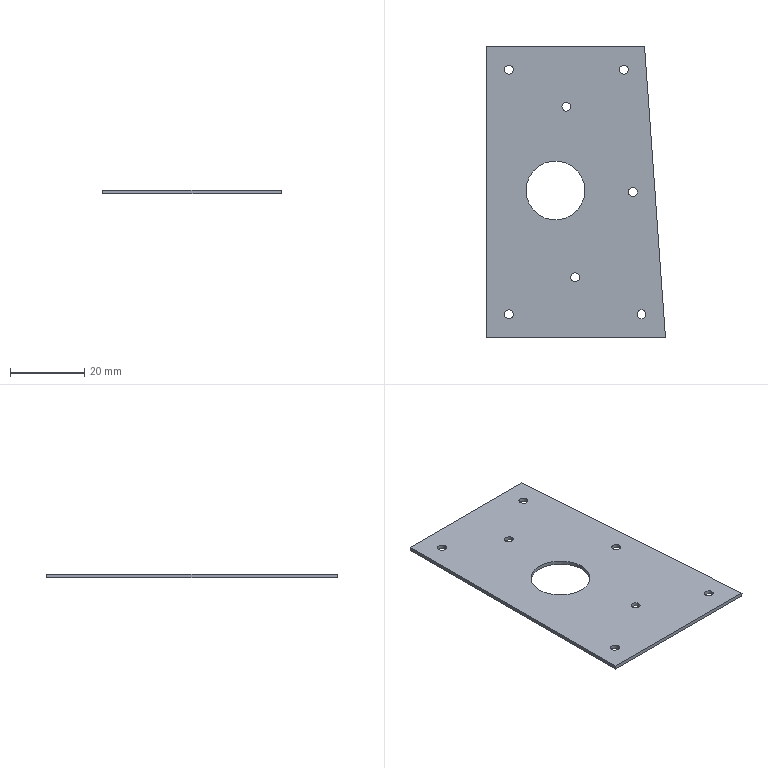Part | SolidWorks | features BaseBody 1 | 1 solid | 22 faces | box 48.271 x 78.4 x 1 mm | volume 3333 mm3 | cylinder 16 | plane 6 | commonest cylinder face diameters 2.4 x14 15.9 x2
STEP:
#1=CARTESIAN_POINT('',(26.55,40.,0.));
#2=VERTEX_POINT('',#1);
#3=CARTESIAN_POINT('',(10.65,40.,0.));
#4=VERTEX_POINT('',#3);
#5=CARTESIAN_POINT('',(18.6,40.,0.));
#6=DIRECTION('',(0.,0.,-1.));
#7=DIRECTION('',(1.,0.,0.));
#8=AXIS2_PLACEMENT_3D('',#5,#6,#7);
#9=CIRCLE('',#8,7.95);
#10=EDGE_CURVE('',#2,#4,#9,.T.);
#11=ORIENTED_EDGE('',*,*,#10,.T.);
#12=CARTESIAN_POINT('',(10.65,40.,1.));
#13=VERTEX_POINT('',#12);
#14=CARTESIAN_POINT('',(10.65,40.,0.));
#15=DIRECTION('',(0.,0.,1.));
#16=VECTOR('',#15,1000.);
#17=LINE('',#14,#16);
#18=EDGE_CURVE('',#4,#13,#17,.T.);
#19=ORIENTED_EDGE('',*,*,#18,.T.);
#20=CARTESIAN_POINT('',(26.55,40.,1.));
#21=VERTEX_POINT('',#20);
#22=CARTESIAN_POINT('',(18.6,40.,1.));
#23=DIRECTION('',(0.,0.,1.));
#24=DIRECTION('',(1.,0.,0.));
#25=AXIS2_PLACEMENT_3D('',#22,#23,#24);
#26=CIRCLE('',#25,7.95);
#27=EDGE_CURVE('',#13,#21,#26,.T.);
#28=ORIENTED_EDGE('',*,*,#27,.T.);
#29=CARTESIAN_POINT('',(26.55,40.,0.));
#30=DIRECTION('',(0.,0.,1.));
#31=VECTOR('',#30,1000.);
#32=LINE('',#29,#31);
#33=EDGE_CURVE('',#2,#21,#32,.T.);
#34=ORIENTED_EDGE('',*,*,#33,.F.);
#35=EDGE_LOOP('',(#11,#19,#28,#34));
#36=FACE_OUTER_BOUND('',#35,.T.);
#37=CARTESIAN_POINT('',(18.6,40.,0.));
#38=DIRECTION('',(0.,0.,1.));
#39=DIRECTION('',(1.,0.,0.));
#40=AXIS2_PLACEMENT_3D('',#37,#38,#39);
#41=CYLINDRICAL_SURFACE('',#40,7.95);
#42=ADVANCED_FACE('',(#36),#41,.F.);
#43=CARTESIAN_POINT('',(4.8,72.6,0.));
#44=VERTEX_POINT('',#43);
#45=CARTESIAN_POINT('',(7.2,72.6,0.));
#46=VERTEX_POINT('',#45);
#47=CARTESIAN_POINT('',(6.,72.6,0.));
#48=DIRECTION('',(0.,0.,1.));
#49=DIRECTION('',(1.,0.,0.));
#50=AXIS2_PLACEMENT_3D('',#47,#48,#49);
#51=CIRCLE('',#50,1.2);
#52=EDGE_CURVE('',#44,#46,#51,.T.);
#53=ORIENTED_EDGE('',*,*,#52,.F.);
#54=CARTESIAN_POINT('',(4.8,72.6,1.));
#55=VERTEX_POINT('',#54);
#56=CARTESIAN_POINT('',(4.8,72.6,0.));
#57=DIRECTION('',(0.,0.,1.));
#58=VECTOR('',#57,1000.);
#59=LINE('',#56,#58);
#60=EDGE_CURVE('',#44,#55,#59,.T.);
#61=ORIENTED_EDGE('',*,*,#60,.T.);
#62=CARTESIAN_POINT('',(7.2,72.6,1.));
#63=VERTEX_POINT('',#62);
#64=CARTESIAN_POINT('',(6.,72.6,1.));
#65=DIRECTION('',(0.,0.,1.));
#66=DIRECTION('',(1.,0.,0.));
#67=AXIS2_PLACEMENT_3D('',#64,#65,#66);
#68=CIRCLE('',#67,1.2);
#69=EDGE_CURVE('',#55,#63,#68,.T.);
#70=ORIENTED_EDGE('',*,*,#69,.T.);
#71=CARTESIAN_POINT('',(7.2,72.6,0.));
#72=DIRECTION('',(0.,0.,1.));
#73=VECTOR('',#72,1000.);
#74=LINE('',#71,#73);
#75=EDGE_CURVE('',#46,#63,#74,.T.);
#76=ORIENTED_EDGE('',*,*,#75,.F.);
#77=EDGE_LOOP('',(#53,#61,#70,#76));
#78=FACE_OUTER_BOUND('',#77,.T.);
#79=CARTESIAN_POINT('',(6.,72.6,0.));
#80=DIRECTION('',(0.,0.,1.));
#81=DIRECTION('',(1.,0.,0.));
#82=AXIS2_PLACEMENT_3D('',#79,#80,#81);
#83=CYLINDRICAL_SURFACE('',#82,1.2);
#84=ADVANCED_FACE('',(#78),#83,.F.);
#85=CARTESIAN_POINT('',(35.859,72.6,0.));
#86=VERTEX_POINT('',#85);
#87=CARTESIAN_POINT('',(38.259,72.6,0.));
#88=VERTEX_POINT('',#87);
#89=CARTESIAN_POINT('',(37.059,72.6,0.));
#90=DIRECTION('',(0.,0.,1.));
#91=DIRECTION('',(1.,0.,0.));
#92=AXIS2_PLACEMENT_3D('',#89,#90,#91);
#93=CIRCLE('',#92,1.2);
#94=EDGE_CURVE('',#86,#88,#93,.T.);
#95=ORIENTED_EDGE('',*,*,#94,.F.);
#96=CARTESIAN_POINT('',(35.859,72.6,1.));
#97=VERTEX_POINT('',#96);
#98=CARTESIAN_POINT('',(35.859,72.6,0.));
#99=DIRECTION('',(0.,0.,1.));
#100=VECTOR('',#99,1000.);
#101=LINE('',#98,#100);
#102=EDGE_CURVE('',#86,#97,#101,.T.);
#103=ORIENTED_EDGE('',*,*,#102,.T.);
#104=CARTESIAN_POINT('',(38.259,72.6,1.));
#105=VERTEX_POINT('',#104);
#106=CARTESIAN_POINT('',(37.059,72.6,1.));
#107=DIRECTION('',(0.,0.,1.));
#108=DIRECTION('',(1.,0.,0.));
#109=AXIS2_PLACEMENT_3D('',#106,#107,#108);
#110=CIRCLE('',#109,1.2);
#111=EDGE_CURVE('',#97,#105,#110,.T.);
#112=ORIENTED_EDGE('',*,*,#111,.T.);
#113=CARTESIAN_POINT('',(38.259,72.6,0.));
#114=DIRECTION('',(0.,0.,1.));
#115=VECTOR('',#114,1000.);
#116=LINE('',#113,#115);
#117=EDGE_CURVE('',#88,#105,#116,.T.);
#118=ORIENTED_EDGE('',*,*,#117,.F.);
#119=EDGE_LOOP('',(#95,#103,#112,#118));
#120=FACE_OUTER_BOUND('',#119,.T.);
#121=CARTESIAN_POINT('',(37.059,72.6,0.));
#122=DIRECTION('',(0.,0.,1.));
#123=DIRECTION('',(1.,0.,0.));
#124=AXIS2_PLACEMENT_3D('',#121,#122,#123);
#125=CYLINDRICAL_SURFACE('',#124,1.2);
#126=ADVANCED_FACE('',(#120),#125,.F.);
#127=CARTESIAN_POINT('',(4.8,6.6,0.));
#128=VERTEX_POINT('',#127);
#129=CARTESIAN_POINT('',(7.2,6.6,0.));
#130=VERTEX_POINT('',#129);
#131=CARTESIAN_POINT('',(6.,6.6,0.));
#132=DIRECTION('',(0.,0.,1.));
#133=DIRECTION('',(1.,0.,0.));
#134=AXIS2_PLACEMENT_3D('',#131,#132,#133);
#135=CIRCLE('',#134,1.2);
#136=EDGE_CURVE('',#128,#130,#135,.T.);
#137=ORIENTED_EDGE('',*,*,#136,.F.);
#138=CARTESIAN_POINT('',(4.8,6.6,1.));
#139=VERTEX_POINT('',#138);
#140=CARTESIAN_POINT('',(4.8,6.6,0.));
#141=DIRECTION('',(0.,0.,1.));
#142=VECTOR('',#141,1000.);
#143=LINE('',#140,#142);
#144=EDGE_CURVE('',#128,#139,#143,.T.);
#145=ORIENTED_EDGE('',*,*,#144,.T.);
#146=CARTESIAN_POINT('',(7.2,6.6,1.));
#147=VERTEX_POINT('',#146);
#148=CARTESIAN_POINT('',(6.,6.6,1.));
#149=DIRECTION('',(0.,0.,1.));
#150=DIRECTION('',(1.,0.,0.));
#151=AXIS2_PLACEMENT_3D('',#148,#149,#150);
#152=CIRCLE('',#151,1.2);
#153=EDGE_CURVE('',#139,#147,#152,.T.);
#154=ORIENTED_EDGE('',*,*,#153,.T.);
#155=CARTESIAN_POINT('',(7.2,6.6,0.));
#156=DIRECTION('',(0.,0.,1.));
#157=VECTOR('',#156,1000.);
#158=LINE('',#155,#157);
#159=EDGE_CURVE('',#130,#147,#158,.T.);
#160=ORIENTED_EDGE('',*,*,#159,.F.);
#161=EDGE_LOOP('',(#137,#145,#154,#160));
#162=FACE_OUTER_BOUND('',#161,.T.);
#163=CARTESIAN_POINT('',(6.,6.6,0.));
#164=DIRECTION('',(0.,0.,1.));
#165=DIRECTION('',(1.,0.,0.));
#166=AXIS2_PLACEMENT_3D('',#163,#164,#165);
#167=CYLINDRICAL_SURFACE('',#166,1.2);
#168=ADVANCED_FACE('',(#162),#167,.F.);
#169=CARTESIAN_POINT('',(40.609,6.6,0.));
#170=VERTEX_POINT('',#169);
#171=CARTESIAN_POINT('',(43.009,6.6,0.));
#172=VERTEX_POINT('',#171);
#173=CARTESIAN_POINT('',(41.809,6.6,0.));
#174=DIRECTION('',(0.,0.,1.));
#175=DIRECTION('',(1.,0.,0.));
#176=AXIS2_PLACEMENT_3D('',#173,#174,#175);
#177=CIRCLE('',#176,1.2);
#178=EDGE_CURVE('',#170,#172,#177,.T.);
#179=ORIENTED_EDGE('',*,*,#178,.F.);
#180=CARTESIAN_POINT('',(40.609,6.6,1.));
#181=VERTEX_POINT('',#180);
#182=CARTESIAN_POINT('',(40.609,6.6,0.));
#183=DIRECTION('',(0.,0.,1.));
#184=VECTOR('',#183,1000.);
#185=LINE('',#182,#184);
#186=EDGE_CURVE('',#170,#181,#185,.T.);
#187=ORIENTED_EDGE('',*,*,#186,.T.);
#188=CARTESIAN_POINT('',(43.009,6.6,1.));
#189=VERTEX_POINT('',#188);
#190=CARTESIAN_POINT('',(41.809,6.6,1.));
#191=DIRECTION('',(0.,0.,1.));
#192=DIRECTION('',(1.,0.,0.));
#193=AXIS2_PLACEMENT_3D('',#190,#191,#192);
#194=CIRCLE('',#193,1.2);
#195=EDGE_CURVE('',#181,#189,#194,.T.);
#196=ORIENTED_EDGE('',*,*,#195,.T.);
#197=CARTESIAN_POINT('',(43.009,6.6,0.));
#198=DIRECTION('',(0.,0.,1.));
#199=VECTOR('',#198,1000.);
#200=LINE('',#197,#199);
#201=EDGE_CURVE('',#172,#189,#200,.T.);
#202=ORIENTED_EDGE('',*,*,#201,.F.);
#203=EDGE_LOOP('',(#179,#187,#196,#202));
#204=FACE_OUTER_BOUND('',#203,.T.);
#205=CARTESIAN_POINT('',(41.809,6.6,0.));
#206=DIRECTION('',(0.,0.,1.));
#207=DIRECTION('',(1.,0.,0.));
#208=AXIS2_PLACEMENT_3D('',#205,#206,#207);
#209=CYLINDRICAL_SURFACE('',#208,1.2);
#210=ADVANCED_FACE('',(#204),#209,.F.);
#211=CARTESIAN_POINT('',(38.234,39.6,0.));
#212=VERTEX_POINT('',#211);
#213=CARTESIAN_POINT('',(40.634,39.6,0.));
#214=VERTEX_POINT('',#213);
#215=CARTESIAN_POINT('',(39.434,39.6,0.));
#216=DIRECTION('',(0.,0.,1.));
#217=DIRECTION('',(1.,0.,0.));
#218=AXIS2_PLACEMENT_3D('',#215,#216,#217);
#219=CIRCLE('',#218,1.2);
#220=EDGE_CURVE('',#212,#214,#219,.T.);
#221=ORIENTED_EDGE('',*,*,#220,.F.);
#222=CARTESIAN_POINT('',(38.234,39.6,1.));
#223=VERTEX_POINT('',#222);
#224=CARTESIAN_POINT('',(38.234,39.6,0.));
#225=DIRECTION('',(0.,0.,1.));
#226=VECTOR('',#225,1000.);
#227=LINE('',#224,#226);
#228=EDGE_CURVE('',#212,#223,#227,.T.);
#229=ORIENTED_EDGE('',*,*,#228,.T.);
#230=CARTESIAN_POINT('',(40.634,39.6,1.));
#231=VERTEX_POINT('',#230);
#232=CARTESIAN_POINT('',(39.434,39.6,1.));
#233=DIRECTION('',(0.,0.,1.));
#234=DIRECTION('',(1.,0.,0.));
#235=AXIS2_PLACEMENT_3D('',#232,#233,#234);
#236=CIRCLE('',#235,1.2);
#237=EDGE_CURVE('',#223,#231,#236,.T.);
#238=ORIENTED_EDGE('',*,*,#237,.T.);
#239=CARTESIAN_POINT('',(40.634,39.6,0.));
#240=DIRECTION('',(0.,0.,1.));
#241=VECTOR('',#240,1000.);
#242=LINE('',#239,#241);
#243=EDGE_CURVE('',#214,#231,#242,.T.);
#244=ORIENTED_EDGE('',*,*,#243,.F.);
#245=EDGE_LOOP('',(#221,#229,#238,#244));
#246=FACE_OUTER_BOUND('',#245,.T.);
#247=CARTESIAN_POINT('',(39.434,39.6,0.));
#248=DIRECTION('',(0.,0.,1.));
#249=DIRECTION('',(1.,0.,0.));
#250=AXIS2_PLACEMENT_3D('',#247,#248,#249);
#251=CYLINDRICAL_SURFACE('',#250,1.2);
#252=ADVANCED_FACE('',(#246),#251,.F.);
#253=CARTESIAN_POINT('',(22.705,16.6,0.));
#254=VERTEX_POINT('',#253);
#255=CARTESIAN_POINT('',(25.105,16.6,0.));
#256=VERTEX_POINT('',#255);
#257=CARTESIAN_POINT('',(23.905,16.6,0.));
#258=DIRECTION('',(0.,0.,1.));
#259=DIRECTION('',(1.,0.,0.));
#260=AXIS2_PLACEMENT_3D('',#257,#258,#259);
#261=CIRCLE('',#260,1.2);
#262=EDGE_CURVE('',#254,#256,#261,.T.);
#263=ORIENTED_EDGE('',*,*,#262,.F.);
#264=CARTESIAN_POINT('',(22.705,16.6,1.));
#265=VERTEX_POINT('',#264);
#266=CARTESIAN_POINT('',(22.705,16.6,0.));
#267=DIRECTION('',(0.,0.,1.));
#268=VECTOR('',#267,1000.);
#269=LINE('',#266,#268);
#270=EDGE_CURVE('',#254,#265,#269,.T.);
#271=ORIENTED_EDGE('',*,*,#270,.T.);
#272=CARTESIAN_POINT('',(25.105,16.6,1.));
#273=VERTEX_POINT('',#272);
#274=CARTESIAN_POINT('',(23.905,16.6,1.));
#275=DIRECTION('',(0.,0.,1.));
#276=DIRECTION('',(1.,0.,0.));
#277=AXIS2_PLACEMENT_3D('',#274,#275,#276);
#278=CIRCLE('',#277,1.2);
#279=EDGE_CURVE('',#265,#273,#278,.T.);
#280=ORIENTED_EDGE('',*,*,#279,.T.);
#281=CARTESIAN_POINT('',(25.105,16.6,0.));
#282=DIRECTION('',(0.,0.,1.));
#283=VECTOR('',#282,1000.);
#284=LINE('',#281,#283);
#285=EDGE_CURVE('',#256,#273,#284,.T.);
#286=ORIENTED_EDGE('',*,*,#285,.F.);
#287=EDGE_LOOP('',(#263,#271,#280,#286));
#288=FACE_OUTER_BOUND('',#287,.T.);
#289=CARTESIAN_POINT('',(23.905,16.6,0.));
#290=DIRECTION('',(0.,0.,1.));
#291=DIRECTION('',(1.,0.,0.));
#292=AXIS2_PLACEMENT_3D('',#289,#290,#291);
#293=CYLINDRICAL_SURFACE('',#292,1.2);
#294=ADVANCED_FACE('',(#288),#293,.F.);
#295=CARTESIAN_POINT('',(20.33,62.6,0.));
#296=VERTEX_POINT('',#295);
#297=CARTESIAN_POINT('',(22.73,62.6,0.));
#298=VERTEX_POINT('',#297);
#299=CARTESIAN_POINT('',(21.53,62.6,0.));
#300=DIRECTION('',(0.,0.,1.));
#301=DIRECTION('',(1.,0.,0.));
#302=AXIS2_PLACEMENT_3D('',#299,#300,#301);
#303=CIRCLE('',#302,1.2);
#304=EDGE_CURVE('',#296,#298,#303,.T.);
#305=ORIENTED_EDGE('',*,*,#304,.F.);
#306=CARTESIAN_POINT('',(20.33,62.6,1.));
#307=VERTEX_POINT('',#306);
#308=CARTESIAN_POINT('',(20.33,62.6,0.));
#309=DIRECTION('',(0.,0.,1.));
#310=VECTOR('',#309,1000.);
#311=LINE('',#308,#310);
#312=EDGE_CURVE('',#296,#307,#311,.T.);
#313=ORIENTED_EDGE('',*,*,#312,.T.);
#314=CARTESIAN_POINT('',(22.73,62.6,1.));
#315=VERTEX_POINT('',#314);
#316=CARTESIAN_POINT('',(21.53,62.6,1.));
#317=DIRECTION('',(0.,0.,1.));
#318=DIRECTION('',(1.,0.,0.));
#319=AXIS2_PLACEMENT_3D('',#316,#317,#318);
#320=CIRCLE('',#319,1.2);
#321=EDGE_CURVE('',#307,#315,#320,.T.);
#322=ORIENTED_EDGE('',*,*,#321,.T.);
#323=CARTESIAN_POINT('',(22.73,62.6,0.));
#324=DIRECTION('',(0.,0.,1.));
#325=VECTOR('',#324,1000.);
#326=LINE('',#323,#325);
#327=EDGE_CURVE('',#298,#315,#326,.T.);
#328=ORIENTED_EDGE('',*,*,#327,.F.);
#329=EDGE_LOOP('',(#305,#313,#322,#328));
#330=FACE_OUTER_BOUND('',#329,.T.);
#331=CARTESIAN_POINT('',(21.53,62.6,0.));
#332=DIRECTION('',(0.,0.,1.));
#333=DIRECTION('',(1.,0.,0.));
#334=AXIS2_PLACEMENT_3D('',#331,#332,#333);
#335=CYLINDRICAL_SURFACE('',#334,1.2);
#336=ADVANCED_FACE('',(#330),#335,.F.);
#337=ORIENTED_EDGE('',*,*,#18,.F.);
#338=CARTESIAN_POINT('',(18.6,40.,0.));
#339=DIRECTION('',(0.,0.,-1.));
#340=DIRECTION('',(1.,0.,0.));
#341=AXIS2_PLACEMENT_3D('',#338,#339,#340);
#342=CIRCLE('',#341,7.95);
#343=EDGE_CURVE('',#4,#2,#342,.T.);
#344=ORIENTED_EDGE('',*,*,#343,.T.);
#345=ORIENTED_EDGE('',*,*,#33,.T.);
#346=CARTESIAN_POINT('',(18.6,40.,1.));
#347=DIRECTION('',(0.,0.,1.));
#348=DIRECTION('',(1.,0.,0.));
#349=AXIS2_PLACEMENT_3D('',#346,#347,#348);
#350=CIRCLE('',#349,7.95);
#351=EDGE_CURVE('',#21,#13,#350,.T.);
#352=ORIENTED_EDGE('',*,*,#351,.T.);
#353=EDGE_LOOP('',(#337,#344,#345,#352));
#354=FACE_OUTER_BOUND('',#353,.T.);
#355=CARTESIAN_POINT('',(18.6,40.,0.));
#356=DIRECTION('',(0.,0.,1.));
#357=DIRECTION('',(1.,0.,0.));
#358=AXIS2_PLACEMENT_3D('',#355,#356,#357);
#359=CYLINDRICAL_SURFACE('',#358,7.95);
#360=ADVANCED_FACE('',(#354),#359,.F.);
#361=CARTESIAN_POINT('',(6.,72.6,1.));
#362=DIRECTION('',(0.,0.,1.));
#363=DIRECTION('',(1.,0.,0.));
#364=AXIS2_PLACEMENT_3D('',#361,#362,#363);
#365=CIRCLE('',#364,1.2);
#366=EDGE_CURVE('',#63,#55,#365,.T.);
#367=ORIENTED_EDGE('',*,*,#366,.F.);
#368=ORIENTED_EDGE('',*,*,#69,.F.);
#369=EDGE_LOOP('',(#367,#368));
#370=FACE_BOUND('',#369,.T.);
#371=CARTESIAN_POINT('',(37.059,72.6,1.));
#372=DIRECTION('',(0.,0.,1.));
#373=DIRECTION('',(1.,0.,0.));
#374=AXIS2_PLACEMENT_3D('',#371,#372,#373);
#375=CIRCLE('',#374,1.2);
#376=EDGE_CURVE('',#105,#97,#375,.T.);
#377=ORIENTED_EDGE('',*,*,#376,.F.);
#378=ORIENTED_EDGE('',*,*,#111,.F.);
#379=EDGE_LOOP('',(#377,#378));
#380=FACE_BOUND('',#379,.T.);
#381=CARTESIAN_POINT('',(6.,6.6,1.));
#382=DIRECTION('',(0.,0.,1.));
#383=DIRECTION('',(1.,0.,0.));
#384=AXIS2_PLACEMENT_3D('',#381,#382,#383);
#385=CIRCLE('',#384,1.2);
#386=EDGE_CURVE('',#147,#139,#385,.T.);
#387=ORIENTED_EDGE('',*,*,#386,.F.);
#388=ORIENTED_EDGE('',*,*,#153,.F.);
#389=EDGE_LOOP('',(#387,#388));
#390=FACE_BOUND('',#389,.T.);
#391=CARTESIAN_POINT('',(41.809,6.6,1.));
#392=DIRECTION('',(0.,0.,1.));
#393=DIRECTION('',(1.,0.,0.));
#394=AXIS2_PLACEMENT_3D('',#391,#392,#393);
#395=CIRCLE('',#394,1.2);
#396=EDGE_CURVE('',#189,#181,#395,.T.);
#397=ORIENTED_EDGE('',*,*,#396,.F.);
#398=ORIENTED_EDGE('',*,*,#195,.F.);
#399=EDGE_LOOP('',(#397,#398));
#400=FACE_BOUND('',#399,.T.);
#401=CARTESIAN_POINT('',(39.434,39.6,1.));
#402=DIRECTION('',(0.,0.,1.));
#403=DIRECTION('',(1.,0.,0.));
#404=AXIS2_PLACEMENT_3D('',#401,#402,#403);
#405=CIRCLE('',#404,1.2);
#406=EDGE_CURVE('',#231,#223,#405,.T.);
#407=ORIENTED_EDGE('',*,*,#406,.F.);
#408=ORIENTED_EDGE('',*,*,#237,.F.);
#409=EDGE_LOOP('',(#407,#408));
#410=FACE_BOUND('',#409,.T.);
#411=CARTESIAN_POINT('',(23.905,16.6,1.));
#412=DIRECTION('',(0.,0.,1.));
#413=DIRECTION('',(1.,0.,0.));
#414=AXIS2_PLACEMENT_3D('',#411,#412,#413);
#415=CIRCLE('',#414,1.2);
#416=EDGE_CURVE('',#273,#265,#415,.T.);
#417=ORIENTED_EDGE('',*,*,#416,.F.);
#418=ORIENTED_EDGE('',*,*,#279,.F.);
#419=EDGE_LOOP('',(#417,#418));
#420=FACE_BOUND('',#419,.T.);
#421=CARTESIAN_POINT('',(21.53,62.6,1.));
#422=DIRECTION('',(0.,0.,1.));
#423=DIRECTION('',(1.,0.,0.));
#424=AXIS2_PLACEMENT_3D('',#421,#422,#423);
#425=CIRCLE('',#424,1.2);
#426=EDGE_CURVE('',#315,#307,#425,.T.);
#427=ORIENTED_EDGE('',*,*,#426,.F.);
#428=ORIENTED_EDGE('',*,*,#321,.F.);
#429=EDGE_LOOP('',(#427,#428));
#430=FACE_BOUND('',#429,.T.);
#431=ORIENTED_EDGE('',*,*,#351,.F.);
#432=ORIENTED_EDGE('',*,*,#27,.F.);
#433=EDGE_LOOP('',(#431,#432));
#434=FACE_BOUND('',#433,.T.);
#435=CARTESIAN_POINT('',(48.271,0.4,1.));
#436=VERTEX_POINT('',#435);
#437=CARTESIAN_POINT('',(0.,0.4,1.));
#438=VERTEX_POINT('',#437);
#439=CARTESIAN_POINT('',(24.28,0.4,1.));
#440=DIRECTION('',(-1.,0.,0.));
#441=VECTOR('',#440,1000.);
#442=LINE('',#439,#441);
#443=EDGE_CURVE('',#436,#438,#442,.T.);
#444=ORIENTED_EDGE('',*,*,#443,.F.);
#445=CARTESIAN_POINT('',(42.629,78.8,1.));
#446=VERTEX_POINT('',#445);
#447=CARTESIAN_POINT('',(42.629,78.8,1.));
#448=DIRECTION('',(0.07178,-0.9974,0.));
#449=VECTOR('',#448,1000.);
#450=LINE('',#447,#449);
#451=EDGE_CURVE('',#446,#436,#450,.T.);
#452=ORIENTED_EDGE('',*,*,#451,.F.);
#453=CARTESIAN_POINT('',(0.,78.8,1.));
#454=VERTEX_POINT('',#453);
#455=CARTESIAN_POINT('',(24.28,78.8,1.));
#456=DIRECTION('',(1.,0.,0.));
#457=VECTOR('',#456,1000.);
#458=LINE('',#455,#457);
#459=EDGE_CURVE('',#454,#446,#458,.T.);
#460=ORIENTED_EDGE('',*,*,#459,.F.);
#461=CARTESIAN_POINT('',(0.,39.6,1.));
#462=DIRECTION('',(0.,1.,0.));
#463=VECTOR('',#462,1000.);
#464=LINE('',#461,#463);
#465=EDGE_CURVE('',#438,#454,#464,.T.);
#466=ORIENTED_EDGE('',*,*,#465,.F.);
#467=EDGE_LOOP('',(#444,#452,#460,#466));
#468=FACE_OUTER_BOUND('',#467,.T.);
#469=CARTESIAN_POINT('',(48.561,0.4,1.));
#470=DIRECTION('',(0.,0.,-1.));
#471=DIRECTION('',(-1.,0.,0.));
#472=AXIS2_PLACEMENT_3D('',#469,#470,#471);
#473=PLANE('',#472);
#474=ADVANCED_FACE('',(#370,#380,#390,#400,#410,#420,#430,#434,#468),#473,.F.);
#475=CARTESIAN_POINT('',(6.,72.6,0.));
#476=DIRECTION('',(0.,0.,1.));
#477=DIRECTION('',(1.,0.,0.));
#478=AXIS2_PLACEMENT_3D('',#475,#476,#477);
#479=CIRCLE('',#478,1.2);
#480=EDGE_CURVE('',#46,#44,#479,.T.);
#481=ORIENTED_EDGE('',*,*,#480,.T.);
#482=ORIENTED_EDGE('',*,*,#52,.T.);
#483=EDGE_LOOP('',(#481,#482));
#484=FACE_BOUND('',#483,.T.);
#485=CARTESIAN_POINT('',(37.059,72.6,0.));
#486=DIRECTION('',(0.,0.,1.));
#487=DIRECTION('',(1.,0.,0.));
#488=AXIS2_PLACEMENT_3D('',#485,#486,#487);
#489=CIRCLE('',#488,1.2);
#490=EDGE_CURVE('',#88,#86,#489,.T.);
#491=ORIENTED_EDGE('',*,*,#490,.T.);
#492=ORIENTED_EDGE('',*,*,#94,.T.);
#493=EDGE_LOOP('',(#491,#492));
#494=FACE_BOUND('',#493,.T.);
#495=CARTESIAN_POINT('',(6.,6.6,0.));
#496=DIRECTION('',(0.,0.,1.));
#497=DIRECTION('',(1.,0.,0.));
#498=AXIS2_PLACEMENT_3D('',#495,#496,#497);
#499=CIRCLE('',#498,1.2);
#500=EDGE_CURVE('',#130,#128,#499,.T.);
#501=ORIENTED_EDGE('',*,*,#500,.T.);
#502=ORIENTED_EDGE('',*,*,#136,.T.);
#503=EDGE_LOOP('',(#501,#502));
#504=FACE_BOUND('',#503,.T.);
#505=CARTESIAN_POINT('',(41.809,6.6,0.));
#506=DIRECTION('',(0.,0.,1.));
#507=DIRECTION('',(1.,0.,0.));
#508=AXIS2_PLACEMENT_3D('',#505,#506,#507);
#509=CIRCLE('',#508,1.2);
#510=EDGE_CURVE('',#172,#170,#509,.T.);
#511=ORIENTED_EDGE('',*,*,#510,.T.);
#512=ORIENTED_EDGE('',*,*,#178,.T.);
#513=EDGE_LOOP('',(#511,#512));
#514=FACE_BOUND('',#513,.T.);
#515=CARTESIAN_POINT('',(39.434,39.6,0.));
#516=DIRECTION('',(0.,0.,1.));
#517=DIRECTION('',(1.,0.,0.));
#518=AXIS2_PLACEMENT_3D('',#515,#516,#517);
#519=CIRCLE('',#518,1.2);
#520=EDGE_CURVE('',#214,#212,#519,.T.);
#521=ORIENTED_EDGE('',*,*,#520,.T.);
#522=ORIENTED_EDGE('',*,*,#220,.T.);
#523=EDGE_LOOP('',(#521,#522));
#524=FACE_BOUND('',#523,.T.);
#525=CARTESIAN_POINT('',(23.905,16.6,0.));
#526=DIRECTION('',(0.,0.,1.));
#527=DIRECTION('',(1.,0.,0.));
#528=AXIS2_PLACEMENT_3D('',#525,#526,#527);
#529=CIRCLE('',#528,1.2);
#530=EDGE_CURVE('',#256,#254,#529,.T.);
#531=ORIENTED_EDGE('',*,*,#530,.T.);
#532=ORIENTED_EDGE('',*,*,#262,.T.);
#533=EDGE_LOOP('',(#531,#532));
#534=FACE_BOUND('',#533,.T.);
#535=CARTESIAN_POINT('',(21.53,62.6,0.));
#536=DIRECTION('',(0.,0.,1.));
#537=DIRECTION('',(1.,0.,0.));
#538=AXIS2_PLACEMENT_3D('',#535,#536,#537);
#539=CIRCLE('',#538,1.2);
#540=EDGE_CURVE('',#298,#296,#539,.T.);
#541=ORIENTED_EDGE('',*,*,#540,.T.);
#542=ORIENTED_EDGE('',*,*,#304,.T.);
#543=EDGE_LOOP('',(#541,#542));
#544=FACE_BOUND('',#543,.T.);
#545=ORIENTED_EDGE('',*,*,#10,.F.);
#546=ORIENTED_EDGE('',*,*,#343,.F.);
#547=EDGE_LOOP('',(#545,#546));
#548=FACE_BOUND('',#547,.T.);
#549=CARTESIAN_POINT('',(0.,78.8,0.));
#550=VERTEX_POINT('',#549);
#551=CARTESIAN_POINT('',(42.629,78.8,0.));
#552=VERTEX_POINT('',#551);
#553=CARTESIAN_POINT('',(24.28,78.8,0.));
#554=DIRECTION('',(1.,0.,0.));
#555=VECTOR('',#554,1000.);
#556=LINE('',#553,#555);
#557=EDGE_CURVE('',#550,#552,#556,.T.);
#558=ORIENTED_EDGE('',*,*,#557,.T.);
#559=CARTESIAN_POINT('',(48.271,0.4,0.));
#560=VERTEX_POINT('',#559);
#561=CARTESIAN_POINT('',(42.629,78.8,0.));
#562=DIRECTION('',(0.07178,-0.9974,0.));
#563=VECTOR('',#562,1000.);
#564=LINE('',#561,#563);
#565=EDGE_CURVE('',#552,#560,#564,.T.);
#566=ORIENTED_EDGE('',*,*,#565,.T.);
#567=CARTESIAN_POINT('',(0.,0.4,0.));
#568=VERTEX_POINT('',#567);
#569=CARTESIAN_POINT('',(24.28,0.4,0.));
#570=DIRECTION('',(-1.,0.,0.));
#571=VECTOR('',#570,1000.);
#572=LINE('',#569,#571);
#573=EDGE_CURVE('',#560,#568,#572,.T.);
#574=ORIENTED_EDGE('',*,*,#573,.T.);
#575=CARTESIAN_POINT('',(0.,39.6,0.));
#576=DIRECTION('',(0.,1.,0.));
#577=VECTOR('',#576,1000.);
#578=LINE('',#575,#577);
#579=EDGE_CURVE('',#568,#550,#578,.T.);
#580=ORIENTED_EDGE('',*,*,#579,.T.);
#581=EDGE_LOOP('',(#558,#566,#574,#580));
#582=FACE_OUTER_BOUND('',#581,.T.);
#583=CARTESIAN_POINT('',(48.561,0.4,0.));
#584=DIRECTION('',(0.,0.,-1.));
#585=DIRECTION('',(-1.,0.,0.));
#586=AXIS2_PLACEMENT_3D('',#583,#584,#585);
#587=PLANE('',#586);
#588=ADVANCED_FACE('',(#484,#494,#504,#514,#524,#534,#544,#548,#582),#587,.T.);
#589=ORIENTED_EDGE('',*,*,#60,.F.);
#590=ORIENTED_EDGE('',*,*,#480,.F.);
#591=ORIENTED_EDGE('',*,*,#75,.T.);
#592=ORIENTED_EDGE('',*,*,#366,.T.);
#593=EDGE_LOOP('',(#589,#590,#591,#592));
#594=FACE_OUTER_BOUND('',#593,.T.);
#595=CARTESIAN_POINT('',(6.,72.6,0.));
#596=DIRECTION('',(0.,0.,1.));
#597=DIRECTION('',(1.,0.,0.));
#598=AXIS2_PLACEMENT_3D('',#595,#596,#597);
#599=CYLINDRICAL_SURFACE('',#598,1.2);
#600=ADVANCED_FACE('',(#594),#599,.F.);
#601=ORIENTED_EDGE('',*,*,#102,.F.);
#602=ORIENTED_EDGE('',*,*,#490,.F.);
#603=ORIENTED_EDGE('',*,*,#117,.T.);
#604=ORIENTED_EDGE('',*,*,#376,.T.);
#605=EDGE_LOOP('',(#601,#602,#603,#604));
#606=FACE_OUTER_BOUND('',#605,.T.);
#607=CARTESIAN_POINT('',(37.059,72.6,0.));
#608=DIRECTION('',(0.,0.,1.));
#609=DIRECTION('',(1.,0.,0.));
#610=AXIS2_PLACEMENT_3D('',#607,#608,#609);
#611=CYLINDRICAL_SURFACE('',#610,1.2);
#612=ADVANCED_FACE('',(#606),#611,.F.);
#613=ORIENTED_EDGE('',*,*,#144,.F.);
#614=ORIENTED_EDGE('',*,*,#500,.F.);
#615=ORIENTED_EDGE('',*,*,#159,.T.);
#616=ORIENTED_EDGE('',*,*,#386,.T.);
#617=EDGE_LOOP('',(#613,#614,#615,#616));
#618=FACE_OUTER_BOUND('',#617,.T.);
#619=CARTESIAN_POINT('',(6.,6.6,0.));
#620=DIRECTION('',(0.,0.,1.));
#621=DIRECTION('',(1.,0.,0.));
#622=AXIS2_PLACEMENT_3D('',#619,#620,#621);
#623=CYLINDRICAL_SURFACE('',#622,1.2);
#624=ADVANCED_FACE('',(#618),#623,.F.);
#625=ORIENTED_EDGE('',*,*,#186,.F.);
#626=ORIENTED_EDGE('',*,*,#510,.F.);
#627=ORIENTED_EDGE('',*,*,#201,.T.);
#628=ORIENTED_EDGE('',*,*,#396,.T.);
#629=EDGE_LOOP('',(#625,#626,#627,#628));
#630=FACE_OUTER_BOUND('',#629,.T.);
#631=CARTESIAN_POINT('',(41.809,6.6,0.));
#632=DIRECTION('',(0.,0.,1.));
#633=DIRECTION('',(1.,0.,0.));
#634=AXIS2_PLACEMENT_3D('',#631,#632,#633);
#635=CYLINDRICAL_SURFACE('',#634,1.2);
#636=ADVANCED_FACE('',(#630),#635,.F.);
#637=ORIENTED_EDGE('',*,*,#228,.F.);
#638=ORIENTED_EDGE('',*,*,#520,.F.);
#639=ORIENTED_EDGE('',*,*,#243,.T.);
#640=ORIENTED_EDGE('',*,*,#406,.T.);
#641=EDGE_LOOP('',(#637,#638,#639,#640));
#642=FACE_OUTER_BOUND('',#641,.T.);
#643=CARTESIAN_POINT('',(39.434,39.6,0.));
#644=DIRECTION('',(0.,0.,1.));
#645=DIRECTION('',(1.,0.,0.));
#646=AXIS2_PLACEMENT_3D('',#643,#644,#645);
#647=CYLINDRICAL_SURFACE('',#646,1.2);
#648=ADVANCED_FACE('',(#642),#647,.F.);
#649=ORIENTED_EDGE('',*,*,#270,.F.);
#650=ORIENTED_EDGE('',*,*,#530,.F.);
#651=ORIENTED_EDGE('',*,*,#285,.T.);
#652=ORIENTED_EDGE('',*,*,#416,.T.);
#653=EDGE_LOOP('',(#649,#650,#651,#652));
#654=FACE_OUTER_BOUND('',#653,.T.);
#655=CARTESIAN_POINT('',(23.905,16.6,0.));
#656=DIRECTION('',(0.,0.,1.));
#657=DIRECTION('',(1.,0.,0.));
#658=AXIS2_PLACEMENT_3D('',#655,#656,#657);
#659=CYLINDRICAL_SURFACE('',#658,1.2);
#660=ADVANCED_FACE('',(#654),#659,.F.);
#661=ORIENTED_EDGE('',*,*,#312,.F.);
#662=ORIENTED_EDGE('',*,*,#540,.F.);
#663=ORIENTED_EDGE('',*,*,#327,.T.);
#664=ORIENTED_EDGE('',*,*,#426,.T.);
#665=EDGE_LOOP('',(#661,#662,#663,#664));
#666=FACE_OUTER_BOUND('',#665,.T.);
#667=CARTESIAN_POINT('',(21.53,62.6,0.));
#668=DIRECTION('',(0.,0.,1.));
#669=DIRECTION('',(1.,0.,0.));
#670=AXIS2_PLACEMENT_3D('',#667,#668,#669);
#671=CYLINDRICAL_SURFACE('',#670,1.2);
#672=ADVANCED_FACE('',(#666),#671,.F.);
#673=CARTESIAN_POINT('',(0.,0.4,0.5));
#674=DIRECTION('',(0.,0.,-1.));
#675=VECTOR('',#674,1000.);
#676=LINE('',#673,#675);
#677=EDGE_CURVE('',#438,#568,#676,.T.);
#678=ORIENTED_EDGE('',*,*,#677,.F.);
#679=ORIENTED_EDGE('',*,*,#465,.T.);
#680=CARTESIAN_POINT('',(0.,78.8,0.5));
#681=DIRECTION('',(0.,0.,1.));
#682=VECTOR('',#681,1000.);
#683=LINE('',#680,#682);
#684=EDGE_CURVE('',#550,#454,#683,.T.);
#685=ORIENTED_EDGE('',*,*,#684,.F.);
#686=ORIENTED_EDGE('',*,*,#579,.F.);
#687=EDGE_LOOP('',(#678,#679,#685,#686));
#688=FACE_OUTER_BOUND('',#687,.T.);
#689=CARTESIAN_POINT('',(0.,0.4,1.));
#690=DIRECTION('',(1.,0.,0.));
#691=DIRECTION('',(0.,0.,-1.));
#692=AXIS2_PLACEMENT_3D('',#689,#690,#691);
#693=PLANE('',#692);
#694=ADVANCED_FACE('',(#688),#693,.F.);
#695=CARTESIAN_POINT('',(48.271,0.4,0.5));
#696=DIRECTION('',(0.,0.,-1.));
#697=VECTOR('',#696,1000.);
#698=LINE('',#695,#697);
#699=EDGE_CURVE('',#436,#560,#698,.T.);
#700=ORIENTED_EDGE('',*,*,#699,.F.);
#701=ORIENTED_EDGE('',*,*,#443,.T.);
#702=ORIENTED_EDGE('',*,*,#677,.T.);
#703=ORIENTED_EDGE('',*,*,#573,.F.);
#704=EDGE_LOOP('',(#700,#701,#702,#703));
#705=FACE_OUTER_BOUND('',#704,.T.);
#706=CARTESIAN_POINT('',(0.,0.4,0.));
#707=DIRECTION('',(0.,1.,0.));
#708=DIRECTION('',(0.,0.,1.));
#709=AXIS2_PLACEMENT_3D('',#706,#707,#708);
#710=PLANE('',#709);
#711=ADVANCED_FACE('',(#705),#710,.F.);
#712=ORIENTED_EDGE('',*,*,#699,.T.);
#713=ORIENTED_EDGE('',*,*,#565,.F.);
#714=CARTESIAN_POINT('',(42.629,78.8,0.5));
#715=DIRECTION('',(0.,0.,-1.));
#716=VECTOR('',#715,1000.);
#717=LINE('',#714,#716);
#718=EDGE_CURVE('',#446,#552,#717,.T.);
#719=ORIENTED_EDGE('',*,*,#718,.F.);
#720=ORIENTED_EDGE('',*,*,#451,.T.);
#721=EDGE_LOOP('',(#712,#713,#719,#720));
#722=FACE_OUTER_BOUND('',#721,.T.);
#723=CARTESIAN_POINT('',(42.629,78.8,0.));
#724=DIRECTION('',(-0.9974,-0.07178,0.));
#725=DIRECTION('',(0.07178,-0.9974,0.));
#726=AXIS2_PLACEMENT_3D('',#723,#724,#725);
#727=PLANE('',#726);
#728=ADVANCED_FACE('',(#722),#727,.F.);
#729=ORIENTED_EDGE('',*,*,#718,.T.);
#730=ORIENTED_EDGE('',*,*,#557,.F.);
#731=ORIENTED_EDGE('',*,*,#684,.T.);
#732=ORIENTED_EDGE('',*,*,#459,.T.);
#733=EDGE_LOOP('',(#729,#730,#731,#732));
#734=FACE_OUTER_BOUND('',#733,.T.);
#735=CARTESIAN_POINT('',(0.,78.8,1.));
#736=DIRECTION('',(0.,-1.,0.));
#737=DIRECTION('',(0.,0.,-1.));
#738=AXIS2_PLACEMENT_3D('',#735,#736,#737);
#739=PLANE('',#738);
#740=ADVANCED_FACE('',(#734),#739,.F.);
#741=CLOSED_SHELL('',(#42,#84,#126,#168,#210,#252,#294,#336,#360,#474,#588,#600,#612,#624,#636,#648,#660,#672,#694,#711,#728,#740));
#742=MANIFOLD_SOLID_BREP('',#741);
#743=CARTESIAN_POINT('',(0.,0.,0.));
#744=DIRECTION('',(0.,0.,1.));
#745=DIRECTION('',(1.,0.,0.));
#746=AXIS2_PLACEMENT_3D('',#743,#744,#745);
#747=(LENGTH_UNIT()NAMED_UNIT(*)SI_UNIT(.MILLI.,.METRE.));
#748=UNCERTAINTY_MEASURE_WITH_UNIT(LENGTH_MEASURE(0.00001),#747,'','');
#749=(NAMED_UNIT(*)PLANE_ANGLE_UNIT()SI_UNIT($,.RADIAN.));
#750=(NAMED_UNIT(*)SI_UNIT($,.STERADIAN.)SOLID_ANGLE_UNIT());
#751=(GEOMETRIC_REPRESENTATION_CONTEXT(3)GLOBAL_UNCERTAINTY_ASSIGNED_CONTEXT((#748))GLOBAL_UNIT_ASSIGNED_CONTEXT((#747,#749,#750))REPRESENTATION_CONTEXT('',''));
#752=ADVANCED_BREP_SHAPE_REPRESENTATION('',(#742,#746),#751);